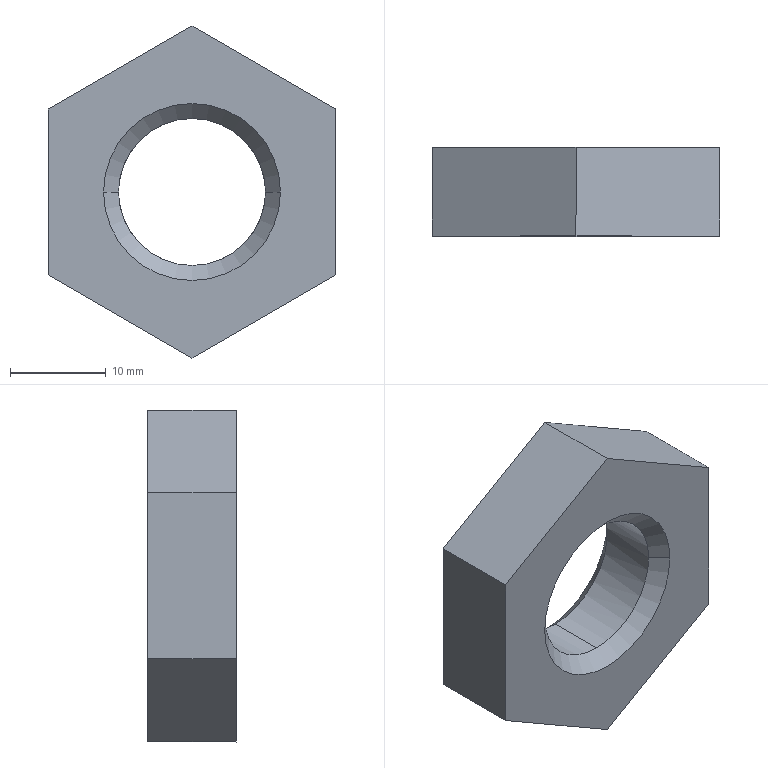Part | SolidWorks | features BaseBody 1 | 1 solid | 14 faces | box 30 x 9.231 x 34.641 mm | volume 5363 mm3 | plane 8 | cone 4 | cylinder 2 | commonest cylinder face diameters 15.339 x2
STEP:
#1=CARTESIAN_POINT('',(57.247,383.17,238.484));
#2=VERTEX_POINT('',#1);
#3=CARTESIAN_POINT('',(57.247,383.17,253.823));
#4=VERTEX_POINT('',#3);
#5=CARTESIAN_POINT('',(57.247,383.17,246.154));
#6=DIRECTION('',(0.,1.,0.));
#7=DIRECTION('',(0.,0.,1.));
#8=AXIS2_PLACEMENT_3D('',#5,#6,#7);
#9=CIRCLE('',#8,7.67);
#10=EDGE_CURVE('',#2,#4,#9,.T.);
#11=ORIENTED_EDGE('',*,*,#10,.F.);
#12=CARTESIAN_POINT('',(57.247,384.731,236.923));
#13=VERTEX_POINT('',#12);
#14=CARTESIAN_POINT('',(57.247,384.731,236.923));
#15=DIRECTION('',(0.,0.7071,-0.7071));
#16=VECTOR('',#15,1000.);
#17=LINE('',#14,#16);
#18=EDGE_CURVE('',#2,#13,#17,.T.);
#19=ORIENTED_EDGE('',*,*,#18,.T.);
#20=CARTESIAN_POINT('',(57.247,384.731,255.385));
#21=VERTEX_POINT('',#20);
#22=CARTESIAN_POINT('',(57.247,384.731,246.154));
#23=DIRECTION('',(0.,1.,0.));
#24=DIRECTION('',(0.,0.,1.));
#25=AXIS2_PLACEMENT_3D('',#22,#23,#24);
#26=CIRCLE('',#25,9.231);
#27=EDGE_CURVE('',#13,#21,#26,.T.);
#28=ORIENTED_EDGE('',*,*,#27,.T.);
#29=CARTESIAN_POINT('',(57.247,384.731,255.385));
#30=DIRECTION('',(0.,0.7071,0.7071));
#31=VECTOR('',#30,1000.);
#32=LINE('',#29,#31);
#33=EDGE_CURVE('',#4,#21,#32,.T.);
#34=ORIENTED_EDGE('',*,*,#33,.F.);
#35=EDGE_LOOP('',(#11,#19,#28,#34));
#36=FACE_OUTER_BOUND('',#35,.T.);
#37=CARTESIAN_POINT('',(57.247,384.731,246.154));
#38=DIRECTION('',(0.,1.,0.));
#39=DIRECTION('',(0.,0.,1.));
#40=AXIS2_PLACEMENT_3D('',#37,#38,#39);
#41=CONICAL_SURFACE('',#40,9.231,0.7854);
#42=ADVANCED_FACE('',(#36),#41,.F.);
#43=ORIENTED_EDGE('',*,*,#10,.T.);
#44=CARTESIAN_POINT('',(57.247,377.061,253.823));
#45=VERTEX_POINT('',#44);
#46=CARTESIAN_POINT('',(57.247,384.731,253.823));
#47=DIRECTION('',(0.,-1.,0.));
#48=VECTOR('',#47,1000.);
#49=LINE('',#46,#48);
#50=EDGE_CURVE('',#4,#45,#49,.T.);
#51=ORIENTED_EDGE('',*,*,#50,.T.);
#52=CARTESIAN_POINT('',(49.577,377.061,246.154));
#53=VERTEX_POINT('',#52);
#54=CARTESIAN_POINT('',(57.247,377.061,246.154));
#55=DIRECTION('',(0.,1.,0.));
#56=DIRECTION('',(0.,0.,-1.));
#57=AXIS2_PLACEMENT_3D('',#54,#55,#56);
#58=CIRCLE('',#57,7.67);
#59=EDGE_CURVE('',#53,#45,#58,.T.);
#60=ORIENTED_EDGE('',*,*,#59,.F.);
#61=CARTESIAN_POINT('',(57.247,377.061,238.484));
#62=VERTEX_POINT('',#61);
#63=CARTESIAN_POINT('',(57.247,377.061,246.154));
#64=DIRECTION('',(0.,1.,0.));
#65=DIRECTION('',(0.,0.,-1.));
#66=AXIS2_PLACEMENT_3D('',#63,#64,#65);
#67=CIRCLE('',#66,7.67);
#68=EDGE_CURVE('',#62,#53,#67,.T.);
#69=ORIENTED_EDGE('',*,*,#68,.F.);
#70=CARTESIAN_POINT('',(57.247,384.731,238.484));
#71=DIRECTION('',(0.,-1.,0.));
#72=VECTOR('',#71,1000.);
#73=LINE('',#70,#72);
#74=EDGE_CURVE('',#2,#62,#73,.T.);
#75=ORIENTED_EDGE('',*,*,#74,.F.);
#76=EDGE_LOOP('',(#43,#51,#60,#69,#75));
#77=FACE_OUTER_BOUND('',#76,.T.);
#78=CARTESIAN_POINT('',(57.247,384.731,246.154));
#79=DIRECTION('',(0.,-1.,0.));
#80=DIRECTION('',(0.,0.,-1.));
#81=AXIS2_PLACEMENT_3D('',#78,#79,#80);
#82=CYLINDRICAL_SURFACE('',#81,7.67);
#83=ADVANCED_FACE('',(#77),#82,.F.);
#84=CARTESIAN_POINT('',(64.916,377.061,246.154));
#85=VERTEX_POINT('',#84);
#86=CARTESIAN_POINT('',(57.247,377.061,246.154));
#87=DIRECTION('',(0.,1.,0.));
#88=DIRECTION('',(0.,0.,-1.));
#89=AXIS2_PLACEMENT_3D('',#86,#87,#88);
#90=CIRCLE('',#89,7.67);
#91=EDGE_CURVE('',#85,#62,#90,.T.);
#92=ORIENTED_EDGE('',*,*,#91,.T.);
#93=ORIENTED_EDGE('',*,*,#68,.T.);
#94=CARTESIAN_POINT('',(48.016,375.5,246.154));
#95=VERTEX_POINT('',#94);
#96=CARTESIAN_POINT('',(48.016,375.5,246.154));
#97=DIRECTION('',(-0.7071,-0.7071,0.));
#98=VECTOR('',#97,1000.);
#99=LINE('',#96,#98);
#100=EDGE_CURVE('',#53,#95,#99,.T.);
#101=ORIENTED_EDGE('',*,*,#100,.T.);
#102=CARTESIAN_POINT('',(66.477,375.5,246.154));
#103=VERTEX_POINT('',#102);
#104=CARTESIAN_POINT('',(57.247,375.5,246.154));
#105=DIRECTION('',(0.,1.,0.));
#106=DIRECTION('',(1.,0.,0.));
#107=AXIS2_PLACEMENT_3D('',#104,#105,#106);
#108=CIRCLE('',#107,9.231);
#109=EDGE_CURVE('',#103,#95,#108,.T.);
#110=ORIENTED_EDGE('',*,*,#109,.F.);
#111=CARTESIAN_POINT('',(66.477,375.5,246.154));
#112=DIRECTION('',(0.7071,-0.7071,0.));
#113=VECTOR('',#112,1000.);
#114=LINE('',#111,#113);
#115=EDGE_CURVE('',#85,#103,#114,.T.);
#116=ORIENTED_EDGE('',*,*,#115,.F.);
#117=EDGE_LOOP('',(#92,#93,#101,#110,#116));
#118=FACE_OUTER_BOUND('',#117,.T.);
#119=CARTESIAN_POINT('',(57.247,375.5,246.154));
#120=DIRECTION('',(0.,-1.,0.));
#121=DIRECTION('',(1.,0.,0.));
#122=AXIS2_PLACEMENT_3D('',#119,#120,#121);
#123=CONICAL_SURFACE('',#122,9.231,0.7854);
#124=ADVANCED_FACE('',(#118),#123,.F.);
#125=CARTESIAN_POINT('',(57.247,384.731,246.154));
#126=DIRECTION('',(0.,1.,0.));
#127=DIRECTION('',(0.,0.,1.));
#128=AXIS2_PLACEMENT_3D('',#125,#126,#127);
#129=CIRCLE('',#128,9.231);
#130=EDGE_CURVE('',#21,#13,#129,.T.);
#131=ORIENTED_EDGE('',*,*,#130,.F.);
#132=ORIENTED_EDGE('',*,*,#27,.F.);
#133=EDGE_LOOP('',(#131,#132));
#134=FACE_BOUND('',#133,.T.);
#135=CARTESIAN_POINT('',(57.247,384.731,263.474));
#136=VERTEX_POINT('',#135);
#137=CARTESIAN_POINT('',(42.247,384.731,254.814));
#138=VERTEX_POINT('',#137);
#139=CARTESIAN_POINT('',(57.247,384.731,263.474));
#140=DIRECTION('',(-0.866,0.,-0.5));
#141=VECTOR('',#140,1000.);
#142=LINE('',#139,#141);
#143=EDGE_CURVE('',#136,#138,#142,.T.);
#144=ORIENTED_EDGE('',*,*,#143,.F.);
#145=CARTESIAN_POINT('',(72.247,384.731,254.814));
#146=VERTEX_POINT('',#145);
#147=CARTESIAN_POINT('',(72.247,384.731,254.814));
#148=DIRECTION('',(-0.866,0.,0.5));
#149=VECTOR('',#148,1000.);
#150=LINE('',#147,#149);
#151=EDGE_CURVE('',#146,#136,#150,.T.);
#152=ORIENTED_EDGE('',*,*,#151,.F.);
#153=CARTESIAN_POINT('',(72.247,384.731,237.494));
#154=VERTEX_POINT('',#153);
#155=CARTESIAN_POINT('',(72.247,384.731,246.154));
#156=DIRECTION('',(0.,0.,1.));
#157=VECTOR('',#156,1000.);
#158=LINE('',#155,#157);
#159=EDGE_CURVE('',#154,#146,#158,.T.);
#160=ORIENTED_EDGE('',*,*,#159,.F.);
#161=CARTESIAN_POINT('',(57.247,384.731,228.833));
#162=VERTEX_POINT('',#161);
#163=CARTESIAN_POINT('',(57.247,384.731,228.833));
#164=DIRECTION('',(0.866,0.,0.5));
#165=VECTOR('',#164,1000.);
#166=LINE('',#163,#165);
#167=EDGE_CURVE('',#162,#154,#166,.T.);
#168=ORIENTED_EDGE('',*,*,#167,.F.);
#169=CARTESIAN_POINT('',(42.247,384.731,237.494));
#170=VERTEX_POINT('',#169);
#171=CARTESIAN_POINT('',(42.247,384.731,237.494));
#172=DIRECTION('',(0.866,0.,-0.5));
#173=VECTOR('',#172,1000.);
#174=LINE('',#171,#173);
#175=EDGE_CURVE('',#170,#162,#174,.T.);
#176=ORIENTED_EDGE('',*,*,#175,.F.);
#177=CARTESIAN_POINT('',(42.247,384.731,246.154));
#178=DIRECTION('',(0.,0.,-1.));
#179=VECTOR('',#178,1000.);
#180=LINE('',#177,#179);
#181=EDGE_CURVE('',#138,#170,#180,.T.);
#182=ORIENTED_EDGE('',*,*,#181,.F.);
#183=EDGE_LOOP('',(#144,#152,#160,#168,#176,#182));
#184=FACE_OUTER_BOUND('',#183,.T.);
#185=CARTESIAN_POINT('',(57.247,384.731,246.154));
#186=DIRECTION('',(0.,-1.,0.));
#187=DIRECTION('',(0.,0.,-1.));
#188=AXIS2_PLACEMENT_3D('',#185,#186,#187);
#189=PLANE('',#188);
#190=ADVANCED_FACE('',(#134,#184),#189,.F.);
#191=ORIENTED_EDGE('',*,*,#18,.F.);
#192=CARTESIAN_POINT('',(57.247,383.17,246.154));
#193=DIRECTION('',(0.,1.,0.));
#194=DIRECTION('',(0.,0.,1.));
#195=AXIS2_PLACEMENT_3D('',#192,#193,#194);
#196=CIRCLE('',#195,7.67);
#197=EDGE_CURVE('',#4,#2,#196,.T.);
#198=ORIENTED_EDGE('',*,*,#197,.F.);
#199=ORIENTED_EDGE('',*,*,#33,.T.);
#200=ORIENTED_EDGE('',*,*,#130,.T.);
#201=EDGE_LOOP('',(#191,#198,#199,#200));
#202=FACE_OUTER_BOUND('',#201,.T.);
#203=CARTESIAN_POINT('',(57.247,384.731,246.154));
#204=DIRECTION('',(0.,1.,0.));
#205=DIRECTION('',(0.,0.,1.));
#206=AXIS2_PLACEMENT_3D('',#203,#204,#205);
#207=CONICAL_SURFACE('',#206,9.231,0.7854);
#208=ADVANCED_FACE('',(#202),#207,.F.);
#209=CARTESIAN_POINT('',(42.247,375.5,254.814));
#210=VERTEX_POINT('',#209);
#211=CARTESIAN_POINT('',(42.247,384.731,254.814));
#212=DIRECTION('',(0.,1.,0.));
#213=VECTOR('',#212,1000.);
#214=LINE('',#211,#213);
#215=EDGE_CURVE('',#210,#138,#214,.T.);
#216=ORIENTED_EDGE('',*,*,#215,.T.);
#217=ORIENTED_EDGE('',*,*,#181,.T.);
#218=CARTESIAN_POINT('',(42.247,375.5,237.494));
#219=VERTEX_POINT('',#218);
#220=CARTESIAN_POINT('',(42.247,384.731,237.494));
#221=DIRECTION('',(0.,-1.,0.));
#222=VECTOR('',#221,1000.);
#223=LINE('',#220,#222);
#224=EDGE_CURVE('',#170,#219,#223,.T.);
#225=ORIENTED_EDGE('',*,*,#224,.T.);
#226=CARTESIAN_POINT('',(42.247,375.5,254.814));
#227=DIRECTION('',(0.,0.,1.));
#228=VECTOR('',#227,1000.);
#229=LINE('',#226,#228);
#230=EDGE_CURVE('',#219,#210,#229,.T.);
#231=ORIENTED_EDGE('',*,*,#230,.T.);
#232=EDGE_LOOP('',(#216,#217,#225,#231));
#233=FACE_OUTER_BOUND('',#232,.T.);
#234=CARTESIAN_POINT('',(42.247,384.731,254.814));
#235=DIRECTION('',(-1.,0.,0.));
#236=DIRECTION('',(0.,0.,1.));
#237=AXIS2_PLACEMENT_3D('',#234,#235,#236);
#238=PLANE('',#237);
#239=ADVANCED_FACE('',(#233),#238,.T.);
#240=CARTESIAN_POINT('',(57.247,375.5,263.474));
#241=VERTEX_POINT('',#240);
#242=CARTESIAN_POINT('',(57.247,384.731,263.474));
#243=DIRECTION('',(0.,1.,0.));
#244=VECTOR('',#243,1000.);
#245=LINE('',#242,#244);
#246=EDGE_CURVE('',#241,#136,#245,.T.);
#247=ORIENTED_EDGE('',*,*,#246,.T.);
#248=ORIENTED_EDGE('',*,*,#143,.T.);
#249=ORIENTED_EDGE('',*,*,#215,.F.);
#250=CARTESIAN_POINT('',(57.247,375.5,263.474));
#251=DIRECTION('',(0.866,0.,0.5));
#252=VECTOR('',#251,1000.);
#253=LINE('',#250,#252);
#254=EDGE_CURVE('',#210,#241,#253,.T.);
#255=ORIENTED_EDGE('',*,*,#254,.T.);
#256=EDGE_LOOP('',(#247,#248,#249,#255));
#257=FACE_OUTER_BOUND('',#256,.T.);
#258=CARTESIAN_POINT('',(57.247,384.731,263.474));
#259=DIRECTION('',(-0.5,0.,0.866));
#260=DIRECTION('',(0.866,0.,0.5));
#261=AXIS2_PLACEMENT_3D('',#258,#259,#260);
#262=PLANE('',#261);
#263=ADVANCED_FACE('',(#257),#262,.T.);
#264=CARTESIAN_POINT('',(72.247,375.5,254.814));
#265=VERTEX_POINT('',#264);
#266=CARTESIAN_POINT('',(72.247,384.731,254.814));
#267=DIRECTION('',(0.,1.,0.));
#268=VECTOR('',#267,1000.);
#269=LINE('',#266,#268);
#270=EDGE_CURVE('',#265,#146,#269,.T.);
#271=ORIENTED_EDGE('',*,*,#270,.T.);
#272=ORIENTED_EDGE('',*,*,#151,.T.);
#273=ORIENTED_EDGE('',*,*,#246,.F.);
#274=CARTESIAN_POINT('',(72.247,375.5,254.814));
#275=DIRECTION('',(0.866,0.,-0.5));
#276=VECTOR('',#275,1000.);
#277=LINE('',#274,#276);
#278=EDGE_CURVE('',#241,#265,#277,.T.);
#279=ORIENTED_EDGE('',*,*,#278,.T.);
#280=EDGE_LOOP('',(#271,#272,#273,#279));
#281=FACE_OUTER_BOUND('',#280,.T.);
#282=CARTESIAN_POINT('',(72.247,384.731,254.814));
#283=DIRECTION('',(0.5,0.,0.866));
#284=DIRECTION('',(0.866,0.,-0.5));
#285=AXIS2_PLACEMENT_3D('',#282,#283,#284);
#286=PLANE('',#285);
#287=ADVANCED_FACE('',(#281),#286,.T.);
#288=CARTESIAN_POINT('',(72.247,375.5,237.494));
#289=VERTEX_POINT('',#288);
#290=CARTESIAN_POINT('',(72.247,384.731,237.494));
#291=DIRECTION('',(0.,1.,0.));
#292=VECTOR('',#291,1000.);
#293=LINE('',#290,#292);
#294=EDGE_CURVE('',#289,#154,#293,.T.);
#295=ORIENTED_EDGE('',*,*,#294,.T.);
#296=ORIENTED_EDGE('',*,*,#159,.T.);
#297=ORIENTED_EDGE('',*,*,#270,.F.);
#298=CARTESIAN_POINT('',(72.247,375.5,237.494));
#299=DIRECTION('',(0.,0.,-1.));
#300=VECTOR('',#299,1000.);
#301=LINE('',#298,#300);
#302=EDGE_CURVE('',#265,#289,#301,.T.);
#303=ORIENTED_EDGE('',*,*,#302,.T.);
#304=EDGE_LOOP('',(#295,#296,#297,#303));
#305=FACE_OUTER_BOUND('',#304,.T.);
#306=CARTESIAN_POINT('',(72.247,384.731,237.494));
#307=DIRECTION('',(1.,0.,0.));
#308=DIRECTION('',(0.,0.,-1.));
#309=AXIS2_PLACEMENT_3D('',#306,#307,#308);
#310=PLANE('',#309);
#311=ADVANCED_FACE('',(#305),#310,.T.);
#312=CARTESIAN_POINT('',(57.247,375.5,228.833));
#313=VERTEX_POINT('',#312);
#314=CARTESIAN_POINT('',(57.247,384.731,228.833));
#315=DIRECTION('',(0.,1.,0.));
#316=VECTOR('',#315,1000.);
#317=LINE('',#314,#316);
#318=EDGE_CURVE('',#313,#162,#317,.T.);
#319=ORIENTED_EDGE('',*,*,#318,.T.);
#320=ORIENTED_EDGE('',*,*,#167,.T.);
#321=ORIENTED_EDGE('',*,*,#294,.F.);
#322=CARTESIAN_POINT('',(57.247,375.5,228.833));
#323=DIRECTION('',(-0.866,0.,-0.5));
#324=VECTOR('',#323,1000.);
#325=LINE('',#322,#324);
#326=EDGE_CURVE('',#289,#313,#325,.T.);
#327=ORIENTED_EDGE('',*,*,#326,.T.);
#328=EDGE_LOOP('',(#319,#320,#321,#327));
#329=FACE_OUTER_BOUND('',#328,.T.);
#330=CARTESIAN_POINT('',(57.247,384.731,228.833));
#331=DIRECTION('',(0.5,0.,-0.866));
#332=DIRECTION('',(-0.866,0.,-0.5));
#333=AXIS2_PLACEMENT_3D('',#330,#331,#332);
#334=PLANE('',#333);
#335=ADVANCED_FACE('',(#329),#334,.T.);
#336=ORIENTED_EDGE('',*,*,#224,.F.);
#337=ORIENTED_EDGE('',*,*,#175,.T.);
#338=ORIENTED_EDGE('',*,*,#318,.F.);
#339=CARTESIAN_POINT('',(42.247,375.5,237.494));
#340=DIRECTION('',(-0.866,0.,0.5));
#341=VECTOR('',#340,1000.);
#342=LINE('',#339,#341);
#343=EDGE_CURVE('',#313,#219,#342,.T.);
#344=ORIENTED_EDGE('',*,*,#343,.T.);
#345=EDGE_LOOP('',(#336,#337,#338,#344));
#346=FACE_OUTER_BOUND('',#345,.T.);
#347=CARTESIAN_POINT('',(42.247,384.731,237.494));
#348=DIRECTION('',(-0.5,0.,-0.866));
#349=DIRECTION('',(-0.866,0.,0.5));
#350=AXIS2_PLACEMENT_3D('',#347,#348,#349);
#351=PLANE('',#350);
#352=ADVANCED_FACE('',(#346),#351,.T.);
#353=ORIENTED_EDGE('',*,*,#50,.F.);
#354=ORIENTED_EDGE('',*,*,#197,.T.);
#355=ORIENTED_EDGE('',*,*,#74,.T.);
#356=ORIENTED_EDGE('',*,*,#91,.F.);
#357=CARTESIAN_POINT('',(57.247,377.061,246.154));
#358=DIRECTION('',(0.,1.,0.));
#359=DIRECTION('',(0.,0.,-1.));
#360=AXIS2_PLACEMENT_3D('',#357,#358,#359);
#361=CIRCLE('',#360,7.67);
#362=EDGE_CURVE('',#45,#85,#361,.T.);
#363=ORIENTED_EDGE('',*,*,#362,.F.);
#364=EDGE_LOOP('',(#353,#354,#355,#356,#363));
#365=FACE_OUTER_BOUND('',#364,.T.);
#366=CARTESIAN_POINT('',(57.247,384.731,246.154));
#367=DIRECTION('',(0.,-1.,0.));
#368=DIRECTION('',(0.,0.,-1.));
#369=AXIS2_PLACEMENT_3D('',#366,#367,#368);
#370=CYLINDRICAL_SURFACE('',#369,7.67);
#371=ADVANCED_FACE('',(#365),#370,.F.);
#372=ORIENTED_EDGE('',*,*,#109,.T.);
#373=CARTESIAN_POINT('',(57.247,375.5,246.154));
#374=DIRECTION('',(0.,1.,0.));
#375=DIRECTION('',(1.,0.,0.));
#376=AXIS2_PLACEMENT_3D('',#373,#374,#375);
#377=CIRCLE('',#376,9.231);
#378=EDGE_CURVE('',#95,#103,#377,.T.);
#379=ORIENTED_EDGE('',*,*,#378,.T.);
#380=EDGE_LOOP('',(#372,#379));
#381=FACE_BOUND('',#380,.T.);
#382=ORIENTED_EDGE('',*,*,#254,.F.);
#383=ORIENTED_EDGE('',*,*,#230,.F.);
#384=ORIENTED_EDGE('',*,*,#343,.F.);
#385=ORIENTED_EDGE('',*,*,#326,.F.);
#386=ORIENTED_EDGE('',*,*,#302,.F.);
#387=ORIENTED_EDGE('',*,*,#278,.F.);
#388=EDGE_LOOP('',(#382,#383,#384,#385,#386,#387));
#389=FACE_OUTER_BOUND('',#388,.T.);
#390=CARTESIAN_POINT('',(57.247,375.5,246.154));
#391=DIRECTION('',(0.,-1.,0.));
#392=DIRECTION('',(0.,0.,-1.));
#393=AXIS2_PLACEMENT_3D('',#390,#391,#392);
#394=PLANE('',#393);
#395=ADVANCED_FACE('',(#381,#389),#394,.T.);
#396=ORIENTED_EDGE('',*,*,#100,.F.);
#397=ORIENTED_EDGE('',*,*,#59,.T.);
#398=ORIENTED_EDGE('',*,*,#362,.T.);
#399=ORIENTED_EDGE('',*,*,#115,.T.);
#400=ORIENTED_EDGE('',*,*,#378,.F.);
#401=EDGE_LOOP('',(#396,#397,#398,#399,#400));
#402=FACE_OUTER_BOUND('',#401,.T.);
#403=CARTESIAN_POINT('',(57.247,375.5,246.154));
#404=DIRECTION('',(0.,-1.,0.));
#405=DIRECTION('',(1.,0.,0.));
#406=AXIS2_PLACEMENT_3D('',#403,#404,#405);
#407=CONICAL_SURFACE('',#406,9.231,0.7854);
#408=ADVANCED_FACE('',(#402),#407,.F.);
#409=CLOSED_SHELL('',(#42,#83,#124,#190,#208,#239,#263,#287,#311,#335,#352,#371,#395,#408));
#410=MANIFOLD_SOLID_BREP('',#409);
#411=CARTESIAN_POINT('',(0.,0.,0.));
#412=DIRECTION('',(0.,0.,1.));
#413=DIRECTION('',(1.,0.,0.));
#414=AXIS2_PLACEMENT_3D('',#411,#412,#413);
#415=(LENGTH_UNIT()NAMED_UNIT(*)SI_UNIT(.MILLI.,.METRE.));
#416=UNCERTAINTY_MEASURE_WITH_UNIT(LENGTH_MEASURE(0.00001),#415,'','');
#417=(NAMED_UNIT(*)PLANE_ANGLE_UNIT()SI_UNIT($,.RADIAN.));
#418=(NAMED_UNIT(*)SI_UNIT($,.STERADIAN.)SOLID_ANGLE_UNIT());
#419=(GEOMETRIC_REPRESENTATION_CONTEXT(3)GLOBAL_UNCERTAINTY_ASSIGNED_CONTEXT((#416))GLOBAL_UNIT_ASSIGNED_CONTEXT((#415,#417,#418))REPRESENTATION_CONTEXT('',''));
#420=ADVANCED_BREP_SHAPE_REPRESENTATION('',(#410,#414),#419);